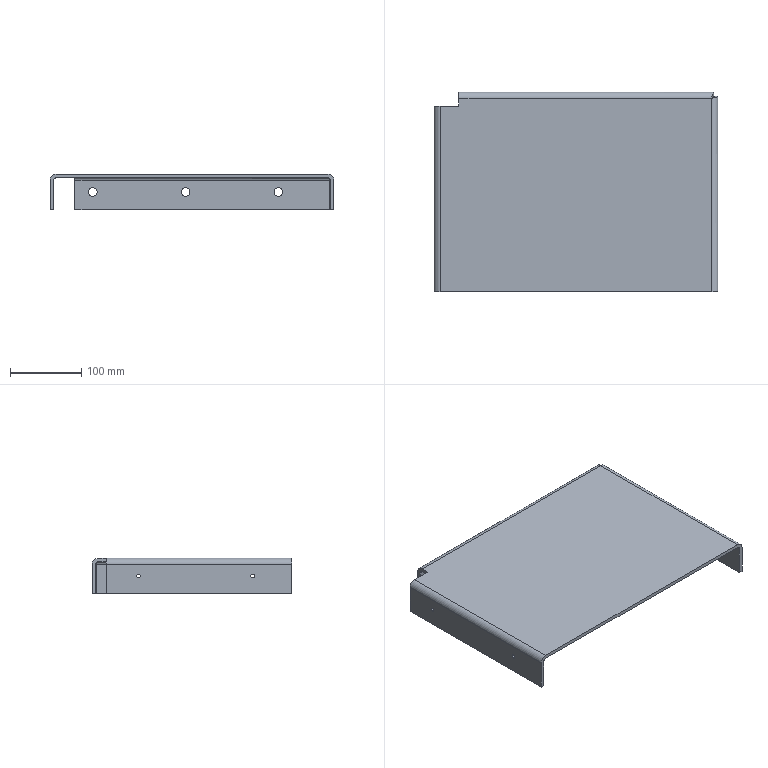Part | STEP file | PN_0020_side plate_default_machined_ | 1 solid | 38 faces | box 398 x 280 x 50 mm | volume 739504 mm3 | cylinder 20 | plane 16 | spline 2 | commonest cylinder face diameters 5 x8 12 x6 8 x3 18 x3